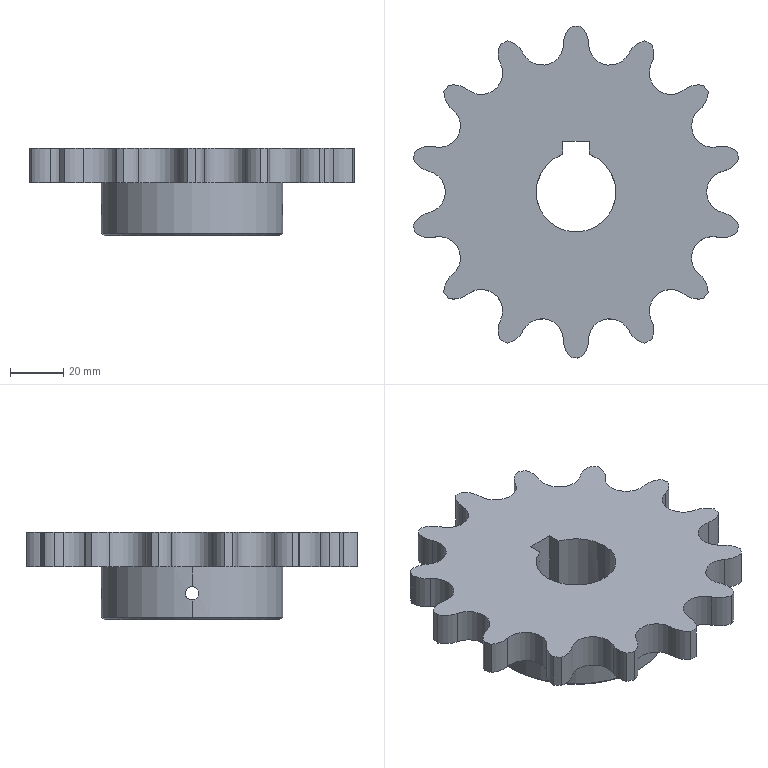Part | STEP file | 链轮-1 (1) | 1 solid | 84 faces | box 122.017 x 124.5 x 33 mm | volume 168369 mm3 | cylinder 76 | plane 6 | cone 2 | commonest cylinder face diameters 17.137 x31 16 x20 124.5 x14 5 x6 30 x3 68 x2